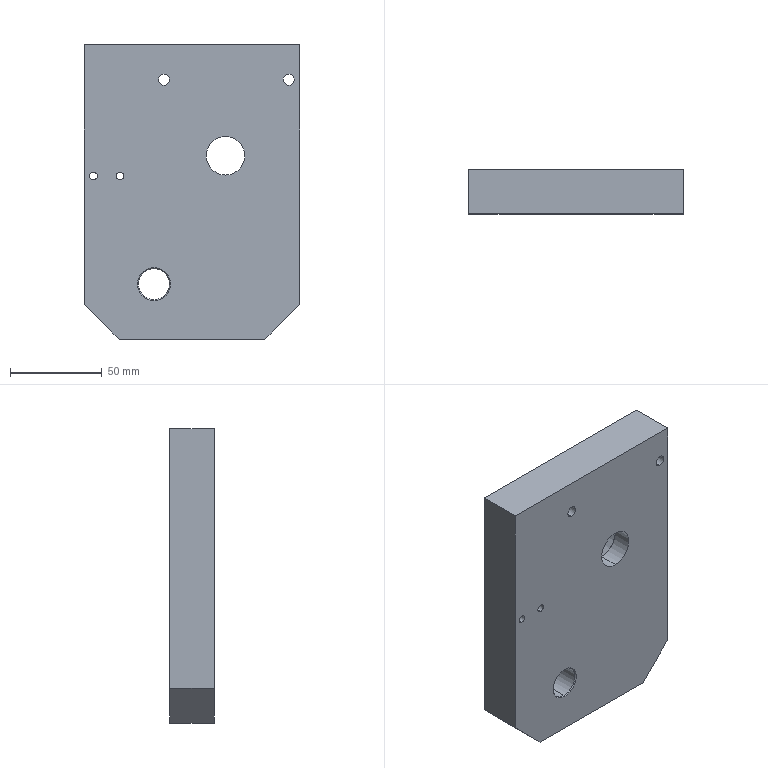Part | SolidWorks | features ICE 4, Chamfer 2, Extrusion 1, HoleWzd 1 | 1 solid | 44 faces | box 117.5 x 24 x 160.5 mm | volume 414919 mm3 | cylinder 17 | cone 14 | plane 13 | commonest cylinder face diameters 4.2 x4 6 x4 11 x3 17 x2 21 x2 40 x2
STEP:
#1=CARTESIAN_POINT('',(52.75,14.5,58.25));
#2=VERTEX_POINT('',#1);
#3=CARTESIAN_POINT('',(52.75,14.5,64.25));
#4=VERTEX_POINT('',#3);
#5=CARTESIAN_POINT('',(52.75,14.5,61.25));
#6=DIRECTION('',(0.,1.,0.));
#7=DIRECTION('',(0.,0.,1.));
#8=AXIS2_PLACEMENT_3D('',#5,#6,#7);
#9=CIRCLE('',#8,3.);
#10=EDGE_CURVE('',#2,#4,#9,.T.);
#11=ORIENTED_EDGE('',*,*,#10,.F.);
#12=CARTESIAN_POINT('',(52.75,15.,57.75));
#13=VERTEX_POINT('',#12);
#14=CARTESIAN_POINT('',(52.75,14.5,58.25));
#15=DIRECTION('',(0.,0.7071,-0.7071));
#16=VECTOR('',#15,1000.);
#17=LINE('',#14,#16);
#18=EDGE_CURVE('',#2,#13,#17,.T.);
#19=ORIENTED_EDGE('',*,*,#18,.T.);
#20=CARTESIAN_POINT('',(52.75,15.,64.75));
#21=VERTEX_POINT('',#20);
#22=CARTESIAN_POINT('',(52.75,15.,61.25));
#23=DIRECTION('',(0.,-1.,0.));
#24=DIRECTION('',(0.,0.,1.));
#25=AXIS2_PLACEMENT_3D('',#22,#23,#24);
#26=CIRCLE('',#25,3.5);
#27=EDGE_CURVE('',#21,#13,#26,.T.);
#28=ORIENTED_EDGE('',*,*,#27,.F.);
#29=CARTESIAN_POINT('',(52.75,14.5,64.25));
#30=DIRECTION('',(0.,0.7071,0.7071));
#31=VECTOR('',#30,1000.);
#32=LINE('',#29,#31);
#33=EDGE_CURVE('',#4,#21,#32,.T.);
#34=ORIENTED_EDGE('',*,*,#33,.F.);
#35=EDGE_LOOP('',(#11,#19,#28,#34));
#36=FACE_OUTER_BOUND('',#35,.T.);
#37=CARTESIAN_POINT('',(52.75,14.5,61.25));
#38=DIRECTION('',(0.,1.,0.));
#39=DIRECTION('',(0.,0.,1.));
#40=AXIS2_PLACEMENT_3D('',#37,#38,#39);
#41=CONICAL_SURFACE('',#40,3.,0.7854);
#42=ADVANCED_FACE('',(#36),#41,.F.);
#43=CARTESIAN_POINT('',(-15.25,15.,55.75));
#44=VERTEX_POINT('',#43);
#45=CARTESIAN_POINT('',(-15.25,15.,66.75));
#46=VERTEX_POINT('',#45);
#47=CARTESIAN_POINT('',(-15.25,15.,61.25));
#48=DIRECTION('',(0.,1.,0.));
#49=DIRECTION('',(0.,0.,1.));
#50=AXIS2_PLACEMENT_3D('',#47,#48,#49);
#51=CIRCLE('',#50,5.5);
#52=EDGE_CURVE('',#44,#46,#51,.T.);
#53=ORIENTED_EDGE('',*,*,#52,.F.);
#54=CARTESIAN_POINT('',(-15.25,24.,55.75));
#55=VERTEX_POINT('',#54);
#56=CARTESIAN_POINT('',(-15.25,15.,55.75));
#57=DIRECTION('',(0.,1.,0.));
#58=VECTOR('',#57,1000.);
#59=LINE('',#56,#58);
#60=EDGE_CURVE('',#44,#55,#59,.T.);
#61=ORIENTED_EDGE('',*,*,#60,.T.);
#62=CARTESIAN_POINT('',(-15.25,24.,66.75));
#63=VERTEX_POINT('',#62);
#64=CARTESIAN_POINT('',(-15.25,24.,61.25));
#65=DIRECTION('',(0.,1.,0.));
#66=DIRECTION('',(0.,0.,1.));
#67=AXIS2_PLACEMENT_3D('',#64,#65,#66);
#68=CIRCLE('',#67,5.5);
#69=EDGE_CURVE('',#55,#63,#68,.T.);
#70=ORIENTED_EDGE('',*,*,#69,.T.);
#71=CARTESIAN_POINT('',(-15.25,15.,66.75));
#72=DIRECTION('',(0.,1.,0.));
#73=VECTOR('',#72,1000.);
#74=LINE('',#71,#73);
#75=EDGE_CURVE('',#46,#63,#74,.T.);
#76=ORIENTED_EDGE('',*,*,#75,.F.);
#77=EDGE_LOOP('',(#53,#61,#70,#76));
#78=FACE_OUTER_BOUND('',#77,.T.);
#79=CARTESIAN_POINT('',(-15.25,15.,61.25));
#80=DIRECTION('',(0.,1.,0.));
#81=DIRECTION('',(0.,0.,1.));
#82=AXIS2_PLACEMENT_3D('',#79,#80,#81);
#83=CYLINDRICAL_SURFACE('',#82,5.5);
#84=ADVANCED_FACE('',(#78),#83,.F.);
#85=CARTESIAN_POINT('',(18.25,23.5,-0.25));
#86=VERTEX_POINT('',#85);
#87=CARTESIAN_POINT('',(18.25,23.5,39.75));
#88=VERTEX_POINT('',#87);
#89=CARTESIAN_POINT('',(18.25,23.5,19.75));
#90=DIRECTION('',(0.,1.,0.));
#91=DIRECTION('',(0.,0.,1.));
#92=AXIS2_PLACEMENT_3D('',#89,#90,#91);
#93=CIRCLE('',#92,20.);
#94=EDGE_CURVE('',#86,#88,#93,.T.);
#95=ORIENTED_EDGE('',*,*,#94,.F.);
#96=CARTESIAN_POINT('',(18.25,24.,-0.75));
#97=VERTEX_POINT('',#96);
#98=CARTESIAN_POINT('',(18.25,23.5,-0.25));
#99=DIRECTION('',(0.,0.7071,-0.7071));
#100=VECTOR('',#99,1000.);
#101=LINE('',#98,#100);
#102=EDGE_CURVE('',#86,#97,#101,.T.);
#103=ORIENTED_EDGE('',*,*,#102,.T.);
#104=CARTESIAN_POINT('',(18.25,24.,40.25));
#105=VERTEX_POINT('',#104);
#106=CARTESIAN_POINT('',(18.25,24.,19.75));
#107=DIRECTION('',(0.,-1.,0.));
#108=DIRECTION('',(0.,0.,1.));
#109=AXIS2_PLACEMENT_3D('',#106,#107,#108);
#110=CIRCLE('',#109,20.5);
#111=EDGE_CURVE('',#105,#97,#110,.T.);
#112=ORIENTED_EDGE('',*,*,#111,.F.);
#113=CARTESIAN_POINT('',(18.25,23.5,39.75));
#114=DIRECTION('',(0.,0.7071,0.7071));
#115=VECTOR('',#114,1000.);
#116=LINE('',#113,#115);
#117=EDGE_CURVE('',#88,#105,#116,.T.);
#118=ORIENTED_EDGE('',*,*,#117,.F.);
#119=EDGE_LOOP('',(#95,#103,#112,#118));
#120=FACE_OUTER_BOUND('',#119,.T.);
#121=CARTESIAN_POINT('',(18.25,23.5,19.75));
#122=DIRECTION('',(0.,1.,0.));
#123=DIRECTION('',(0.,0.,1.));
#124=AXIS2_PLACEMENT_3D('',#121,#122,#123);
#125=CONICAL_SURFACE('',#124,20.,0.7854);
#126=ADVANCED_FACE('',(#120),#125,.F.);
#127=CARTESIAN_POINT('',(18.25,10.5,9.25));
#128=VERTEX_POINT('',#127);
#129=CARTESIAN_POINT('',(18.25,10.5,30.25));
#130=VERTEX_POINT('',#129);
#131=CARTESIAN_POINT('',(18.25,10.5,19.75));
#132=DIRECTION('',(0.,1.,0.));
#133=DIRECTION('',(0.,0.,1.));
#134=AXIS2_PLACEMENT_3D('',#131,#132,#133);
#135=CIRCLE('',#134,10.5);
#136=EDGE_CURVE('',#128,#130,#135,.T.);
#137=ORIENTED_EDGE('',*,*,#136,.F.);
#138=CARTESIAN_POINT('',(18.25,11.,8.75));
#139=VERTEX_POINT('',#138);
#140=CARTESIAN_POINT('',(18.25,10.5,9.25));
#141=DIRECTION('',(0.,0.7071,-0.7071));
#142=VECTOR('',#141,1000.);
#143=LINE('',#140,#142);
#144=EDGE_CURVE('',#128,#139,#143,.T.);
#145=ORIENTED_EDGE('',*,*,#144,.T.);
#146=CARTESIAN_POINT('',(18.25,11.,30.75));
#147=VERTEX_POINT('',#146);
#148=CARTESIAN_POINT('',(18.25,11.,19.75));
#149=DIRECTION('',(0.,-1.,0.));
#150=DIRECTION('',(0.,0.,1.));
#151=AXIS2_PLACEMENT_3D('',#148,#149,#150);
#152=CIRCLE('',#151,11.);
#153=EDGE_CURVE('',#147,#139,#152,.T.);
#154=ORIENTED_EDGE('',*,*,#153,.F.);
#155=CARTESIAN_POINT('',(18.25,10.5,30.25));
#156=DIRECTION('',(0.,0.7071,0.7071));
#157=VECTOR('',#156,1000.);
#158=LINE('',#155,#157);
#159=EDGE_CURVE('',#130,#147,#158,.T.);
#160=ORIENTED_EDGE('',*,*,#159,.F.);
#161=EDGE_LOOP('',(#137,#145,#154,#160));
#162=FACE_OUTER_BOUND('',#161,.T.);
#163=CARTESIAN_POINT('',(18.25,10.5,19.75));
#164=DIRECTION('',(0.,1.,0.));
#165=DIRECTION('',(0.,0.,1.));
#166=AXIS2_PLACEMENT_3D('',#163,#164,#165);
#167=CONICAL_SURFACE('',#166,10.5,0.7854);
#168=ADVANCED_FACE('',(#162),#167,.F.);
#169=CARTESIAN_POINT('',(-20.75,23.5,-58.75));
#170=VERTEX_POINT('',#169);
#171=CARTESIAN_POINT('',(-20.75,23.5,-41.75));
#172=VERTEX_POINT('',#171);
#173=CARTESIAN_POINT('',(-20.75,23.5,-50.25));
#174=DIRECTION('',(0.,1.,0.));
#175=DIRECTION('',(0.,0.,1.));
#176=AXIS2_PLACEMENT_3D('',#173,#174,#175);
#177=CIRCLE('',#176,8.5);
#178=EDGE_CURVE('',#170,#172,#177,.T.);
#179=ORIENTED_EDGE('',*,*,#178,.F.);
#180=CARTESIAN_POINT('',(-20.75,24.,-59.25));
#181=VERTEX_POINT('',#180);
#182=CARTESIAN_POINT('',(-20.75,23.5,-58.75));
#183=DIRECTION('',(0.,0.7071,-0.7071));
#184=VECTOR('',#183,1000.);
#185=LINE('',#182,#184);
#186=EDGE_CURVE('',#170,#181,#185,.T.);
#187=ORIENTED_EDGE('',*,*,#186,.T.);
#188=CARTESIAN_POINT('',(-20.75,24.,-41.25));
#189=VERTEX_POINT('',#188);
#190=CARTESIAN_POINT('',(-20.75,24.,-50.25));
#191=DIRECTION('',(0.,-1.,0.));
#192=DIRECTION('',(0.,0.,1.));
#193=AXIS2_PLACEMENT_3D('',#190,#191,#192);
#194=CIRCLE('',#193,9.);
#195=EDGE_CURVE('',#189,#181,#194,.T.);
#196=ORIENTED_EDGE('',*,*,#195,.F.);
#197=CARTESIAN_POINT('',(-20.75,23.5,-41.75));
#198=DIRECTION('',(0.,0.7071,0.7071));
#199=VECTOR('',#198,1000.);
#200=LINE('',#197,#199);
#201=EDGE_CURVE('',#172,#189,#200,.T.);
#202=ORIENTED_EDGE('',*,*,#201,.F.);
#203=EDGE_LOOP('',(#179,#187,#196,#202));
#204=FACE_OUTER_BOUND('',#203,.T.);
#205=CARTESIAN_POINT('',(-20.75,23.5,-50.25));
#206=DIRECTION('',(0.,1.,0.));
#207=DIRECTION('',(0.,0.,1.));
#208=AXIS2_PLACEMENT_3D('',#205,#206,#207);
#209=CONICAL_SURFACE('',#208,8.5,0.7854);
#210=ADVANCED_FACE('',(#204),#209,.F.);
#211=CARTESIAN_POINT('',(-20.75,0.5,-41.75));
#212=VERTEX_POINT('',#211);
#213=CARTESIAN_POINT('',(-20.75,0.5,-58.75));
#214=VERTEX_POINT('',#213);
#215=CARTESIAN_POINT('',(-20.75,0.5,-50.25));
#216=DIRECTION('',(0.,-1.,0.));
#217=DIRECTION('',(0.,0.,1.));
#218=AXIS2_PLACEMENT_3D('',#215,#216,#217);
#219=CIRCLE('',#218,8.5);
#220=EDGE_CURVE('',#212,#214,#219,.T.);
#221=ORIENTED_EDGE('',*,*,#220,.F.);
#222=CARTESIAN_POINT('',(-20.75,0.,-41.25));
#223=VERTEX_POINT('',#222);
#224=CARTESIAN_POINT('',(-20.75,0.,-41.25));
#225=DIRECTION('',(0.,-0.7071,0.7071));
#226=VECTOR('',#225,1000.);
#227=LINE('',#224,#226);
#228=EDGE_CURVE('',#212,#223,#227,.T.);
#229=ORIENTED_EDGE('',*,*,#228,.T.);
#230=CARTESIAN_POINT('',(-20.75,0.,-59.25));
#231=VERTEX_POINT('',#230);
#232=CARTESIAN_POINT('',(-20.75,0.,-50.25));
#233=DIRECTION('',(0.,1.,0.));
#234=DIRECTION('',(0.,0.,1.));
#235=AXIS2_PLACEMENT_3D('',#232,#233,#234);
#236=CIRCLE('',#235,9.);
#237=EDGE_CURVE('',#231,#223,#236,.T.);
#238=ORIENTED_EDGE('',*,*,#237,.F.);
#239=CARTESIAN_POINT('',(-20.75,0.,-59.25));
#240=DIRECTION('',(0.,-0.7071,-0.7071));
#241=VECTOR('',#240,1000.);
#242=LINE('',#239,#241);
#243=EDGE_CURVE('',#214,#231,#242,.T.);
#244=ORIENTED_EDGE('',*,*,#243,.F.);
#245=EDGE_LOOP('',(#221,#229,#238,#244));
#246=FACE_OUTER_BOUND('',#245,.T.);
#247=CARTESIAN_POINT('',(-20.75,0.,-50.25));
#248=DIRECTION('',(0.,-1.,0.));
#249=DIRECTION('',(0.,0.,-1.));
#250=AXIS2_PLACEMENT_3D('',#247,#248,#249);
#251=CONICAL_SURFACE('',#250,9.,0.7854);
#252=ADVANCED_FACE('',(#246),#251,.F.);
#253=CARTESIAN_POINT('',(-53.75,23.575,6.65));
#254=VERTEX_POINT('',#253);
#255=CARTESIAN_POINT('',(-53.75,23.575,10.85));
#256=VERTEX_POINT('',#255);
#257=CARTESIAN_POINT('',(-53.75,23.575,8.75));
#258=DIRECTION('',(0.,1.,0.));
#259=DIRECTION('',(0.,0.,1.));
#260=AXIS2_PLACEMENT_3D('',#257,#258,#259);
#261=CIRCLE('',#260,2.1);
#262=EDGE_CURVE('',#254,#256,#261,.T.);
#263=ORIENTED_EDGE('',*,*,#262,.F.);
#264=CARTESIAN_POINT('',(-53.75,24.,6.225));
#265=VERTEX_POINT('',#264);
#266=CARTESIAN_POINT('',(-53.75,24.,6.225));
#267=DIRECTION('',(0.,0.7071,-0.7071));
#268=VECTOR('',#267,1000.);
#269=LINE('',#266,#268);
#270=EDGE_CURVE('',#254,#265,#269,.T.);
#271=ORIENTED_EDGE('',*,*,#270,.T.);
#272=CARTESIAN_POINT('',(-53.75,24.,11.275));
#273=VERTEX_POINT('',#272);
#274=CARTESIAN_POINT('',(-53.75,24.,8.75));
#275=DIRECTION('',(0.,1.,0.));
#276=DIRECTION('',(0.,0.,1.));
#277=AXIS2_PLACEMENT_3D('',#274,#275,#276);
#278=CIRCLE('',#277,2.525);
#279=EDGE_CURVE('',#265,#273,#278,.T.);
#280=ORIENTED_EDGE('',*,*,#279,.T.);
#281=CARTESIAN_POINT('',(-53.75,24.,11.275));
#282=DIRECTION('',(0.,0.7071,0.7071));
#283=VECTOR('',#282,1000.);
#284=LINE('',#281,#283);
#285=EDGE_CURVE('',#256,#273,#284,.T.);
#286=ORIENTED_EDGE('',*,*,#285,.F.);
#287=EDGE_LOOP('',(#263,#271,#280,#286));
#288=FACE_OUTER_BOUND('',#287,.T.);
#289=CARTESIAN_POINT('',(-53.75,24.,8.75));
#290=DIRECTION('',(0.,1.,0.));
#291=DIRECTION('',(0.,0.,1.));
#292=AXIS2_PLACEMENT_3D('',#289,#290,#291);
#293=CONICAL_SURFACE('',#292,2.525,0.7854);
#294=ADVANCED_FACE('',(#288),#293,.F.);
#295=CARTESIAN_POINT('',(-53.75,0.,6.65));
#296=VERTEX_POINT('',#295);
#297=CARTESIAN_POINT('',(-53.75,0.,10.85));
#298=VERTEX_POINT('',#297);
#299=CARTESIAN_POINT('',(-53.75,0.,8.75));
#300=DIRECTION('',(0.,1.,0.));
#301=DIRECTION('',(0.,0.,1.));
#302=AXIS2_PLACEMENT_3D('',#299,#300,#301);
#303=CIRCLE('',#302,2.1);
#304=EDGE_CURVE('',#296,#298,#303,.T.);
#305=ORIENTED_EDGE('',*,*,#304,.F.);
#306=CARTESIAN_POINT('',(-53.75,24.,6.65));
#307=DIRECTION('',(0.,1.,0.));
#308=VECTOR('',#307,1000.);
#309=LINE('',#306,#308);
#310=EDGE_CURVE('',#296,#254,#309,.T.);
#311=ORIENTED_EDGE('',*,*,#310,.T.);
#312=ORIENTED_EDGE('',*,*,#262,.T.);
#313=CARTESIAN_POINT('',(-53.75,24.,10.85));
#314=DIRECTION('',(0.,1.,0.));
#315=VECTOR('',#314,1000.);
#316=LINE('',#313,#315);
#317=EDGE_CURVE('',#298,#256,#316,.T.);
#318=ORIENTED_EDGE('',*,*,#317,.F.);
#319=EDGE_LOOP('',(#305,#311,#312,#318));
#320=FACE_OUTER_BOUND('',#319,.T.);
#321=CARTESIAN_POINT('',(-53.75,24.,8.75));
#322=DIRECTION('',(0.,1.,0.));
#323=DIRECTION('',(0.,0.,1.));
#324=AXIS2_PLACEMENT_3D('',#321,#322,#323);
#325=CYLINDRICAL_SURFACE('',#324,2.1);
#326=ADVANCED_FACE('',(#320),#325,.F.);
#327=CARTESIAN_POINT('',(-39.25,23.575,6.65));
#328=VERTEX_POINT('',#327);
#329=CARTESIAN_POINT('',(-39.25,23.575,10.85));
#330=VERTEX_POINT('',#329);
#331=CARTESIAN_POINT('',(-39.25,23.575,8.75));
#332=DIRECTION('',(0.,1.,0.));
#333=DIRECTION('',(0.,0.,1.));
#334=AXIS2_PLACEMENT_3D('',#331,#332,#333);
#335=CIRCLE('',#334,2.1);
#336=EDGE_CURVE('',#328,#330,#335,.T.);
#337=ORIENTED_EDGE('',*,*,#336,.F.);
#338=CARTESIAN_POINT('',(-39.25,24.,6.225));
#339=VERTEX_POINT('',#338);
#340=CARTESIAN_POINT('',(-39.25,24.,6.225));
#341=DIRECTION('',(0.,0.7071,-0.7071));
#342=VECTOR('',#341,1000.);
#343=LINE('',#340,#342);
#344=EDGE_CURVE('',#328,#339,#343,.T.);
#345=ORIENTED_EDGE('',*,*,#344,.T.);
#346=CARTESIAN_POINT('',(-39.25,24.,11.275));
#347=VERTEX_POINT('',#346);
#348=CARTESIAN_POINT('',(-39.25,24.,8.75));
#349=DIRECTION('',(0.,1.,0.));
#350=DIRECTION('',(0.,0.,1.));
#351=AXIS2_PLACEMENT_3D('',#348,#349,#350);
#352=CIRCLE('',#351,2.525);
#353=EDGE_CURVE('',#339,#347,#352,.T.);
#354=ORIENTED_EDGE('',*,*,#353,.T.);
#355=CARTESIAN_POINT('',(-39.25,24.,11.275));
#356=DIRECTION('',(0.,0.7071,0.7071));
#357=VECTOR('',#356,1000.);
#358=LINE('',#355,#357);
#359=EDGE_CURVE('',#330,#347,#358,.T.);
#360=ORIENTED_EDGE('',*,*,#359,.F.);
#361=EDGE_LOOP('',(#337,#345,#354,#360));
#362=FACE_OUTER_BOUND('',#361,.T.);
#363=CARTESIAN_POINT('',(-39.25,24.,8.75));
#364=DIRECTION('',(0.,1.,0.));
#365=DIRECTION('',(0.,0.,1.));
#366=AXIS2_PLACEMENT_3D('',#363,#364,#365);
#367=CONICAL_SURFACE('',#366,2.525,0.7854);
#368=ADVANCED_FACE('',(#362),#367,.F.);
#369=CARTESIAN_POINT('',(-39.25,0.,6.65));
#370=VERTEX_POINT('',#369);
#371=CARTESIAN_POINT('',(-39.25,0.,10.85));
#372=VERTEX_POINT('',#371);
#373=CARTESIAN_POINT('',(-39.25,0.,8.75));
#374=DIRECTION('',(0.,1.,0.));
#375=DIRECTION('',(0.,0.,1.));
#376=AXIS2_PLACEMENT_3D('',#373,#374,#375);
#377=CIRCLE('',#376,2.1);
#378=EDGE_CURVE('',#370,#372,#377,.T.);
#379=ORIENTED_EDGE('',*,*,#378,.F.);
#380=CARTESIAN_POINT('',(-39.25,24.,6.65));
#381=DIRECTION('',(0.,1.,0.));
#382=VECTOR('',#381,1000.);
#383=LINE('',#380,#382);
#384=EDGE_CURVE('',#370,#328,#383,.T.);
#385=ORIENTED_EDGE('',*,*,#384,.T.);
#386=ORIENTED_EDGE('',*,*,#336,.T.);
#387=CARTESIAN_POINT('',(-39.25,24.,10.85));
#388=DIRECTION('',(0.,1.,0.));
#389=VECTOR('',#388,1000.);
#390=LINE('',#387,#389);
#391=EDGE_CURVE('',#372,#330,#390,.T.);
#392=ORIENTED_EDGE('',*,*,#391,.F.);
#393=EDGE_LOOP('',(#379,#385,#386,#392));
#394=FACE_OUTER_BOUND('',#393,.T.);
#395=CARTESIAN_POINT('',(-39.25,24.,8.75));
#396=DIRECTION('',(0.,1.,0.));
#397=DIRECTION('',(0.,0.,1.));
#398=AXIS2_PLACEMENT_3D('',#395,#396,#397);
#399=CYLINDRICAL_SURFACE('',#398,2.1);
#400=ADVANCED_FACE('',(#394),#399,.F.);
#401=CARTESIAN_POINT('',(18.25,0.,9.25));
#402=VERTEX_POINT('',#401);
#403=CARTESIAN_POINT('',(18.25,0.,30.25));
#404=VERTEX_POINT('',#403);
#405=CARTESIAN_POINT('',(18.25,0.,19.75));
#406=DIRECTION('',(0.,1.,0.));
#407=DIRECTION('',(0.,0.,1.));
#408=AXIS2_PLACEMENT_3D('',#405,#406,#407);
#409=CIRCLE('',#408,10.5);
#410=EDGE_CURVE('',#402,#404,#409,.T.);
#411=ORIENTED_EDGE('',*,*,#410,.F.);
#412=CARTESIAN_POINT('',(18.25,0.,9.25));
#413=DIRECTION('',(0.,1.,0.));
#414=VECTOR('',#413,1000.);
#415=LINE('',#412,#414);
#416=EDGE_CURVE('',#402,#128,#415,.T.);
#417=ORIENTED_EDGE('',*,*,#416,.T.);
#418=ORIENTED_EDGE('',*,*,#136,.T.);
#419=CARTESIAN_POINT('',(18.25,0.,30.25));
#420=DIRECTION('',(0.,1.,0.));
#421=VECTOR('',#420,1000.);
#422=LINE('',#419,#421);
#423=EDGE_CURVE('',#404,#130,#422,.T.);
#424=ORIENTED_EDGE('',*,*,#423,.F.);
#425=EDGE_LOOP('',(#411,#417,#418,#424));
#426=FACE_OUTER_BOUND('',#425,.T.);
#427=CARTESIAN_POINT('',(18.25,0.,19.75));
#428=DIRECTION('',(0.,1.,0.));
#429=DIRECTION('',(0.,0.,1.));
#430=AXIS2_PLACEMENT_3D('',#427,#428,#429);
#431=CYLINDRICAL_SURFACE('',#430,10.5);
#432=ADVANCED_FACE('',(#426),#431,.F.);
#433=ORIENTED_EDGE('',*,*,#220,.T.);
#434=CARTESIAN_POINT('',(-20.75,11.,-58.75));
#435=DIRECTION('',(0.,1.,0.));
#436=VECTOR('',#435,1000.);
#437=LINE('',#434,#436);
#438=EDGE_CURVE('',#214,#170,#437,.T.);
#439=ORIENTED_EDGE('',*,*,#438,.T.);
#440=ORIENTED_EDGE('',*,*,#178,.T.);
#441=CARTESIAN_POINT('',(-20.75,11.,-41.75));
#442=DIRECTION('',(0.,1.,0.));
#443=VECTOR('',#442,1000.);
#444=LINE('',#441,#443);
#445=EDGE_CURVE('',#212,#172,#444,.T.);
#446=ORIENTED_EDGE('',*,*,#445,.F.);
#447=EDGE_LOOP('',(#433,#439,#440,#446));
#448=FACE_OUTER_BOUND('',#447,.T.);
#449=CARTESIAN_POINT('',(-20.75,11.,-50.25));
#450=DIRECTION('',(0.,1.,0.));
#451=DIRECTION('',(0.,0.,1.));
#452=AXIS2_PLACEMENT_3D('',#449,#450,#451);
#453=CYLINDRICAL_SURFACE('',#452,8.5);
#454=ADVANCED_FACE('',(#448),#453,.F.);
#455=CARTESIAN_POINT('',(18.25,11.,-0.25));
#456=VERTEX_POINT('',#455);
#457=CARTESIAN_POINT('',(18.25,11.,39.75));
#458=VERTEX_POINT('',#457);
#459=CARTESIAN_POINT('',(18.25,11.,19.75));
#460=DIRECTION('',(0.,1.,0.));
#461=DIRECTION('',(0.,0.,1.));
#462=AXIS2_PLACEMENT_3D('',#459,#460,#461);
#463=CIRCLE('',#462,20.);
#464=EDGE_CURVE('',#456,#458,#463,.T.);
#465=ORIENTED_EDGE('',*,*,#464,.F.);
#466=CARTESIAN_POINT('',(18.25,11.,-0.25));
#467=DIRECTION('',(0.,1.,0.));
#468=VECTOR('',#467,1000.);
#469=LINE('',#466,#468);
#470=EDGE_CURVE('',#456,#86,#469,.T.);
#471=ORIENTED_EDGE('',*,*,#470,.T.);
#472=ORIENTED_EDGE('',*,*,#94,.T.);
#473=CARTESIAN_POINT('',(18.25,11.,39.75));
#474=DIRECTION('',(0.,1.,0.));
#475=VECTOR('',#474,1000.);
#476=LINE('',#473,#475);
#477=EDGE_CURVE('',#458,#88,#476,.T.);
#478=ORIENTED_EDGE('',*,*,#477,.F.);
#479=EDGE_LOOP('',(#465,#471,#472,#478));
#480=FACE_OUTER_BOUND('',#479,.T.);
#481=CARTESIAN_POINT('',(18.25,11.,19.75));
#482=DIRECTION('',(0.,1.,0.));
#483=DIRECTION('',(0.,0.,1.));
#484=AXIS2_PLACEMENT_3D('',#481,#482,#483);
#485=CYLINDRICAL_SURFACE('',#484,20.);
#486=ADVANCED_FACE('',(#480),#485,.F.);
#487=CARTESIAN_POINT('',(52.75,0.,58.25));
#488=VERTEX_POINT('',#487);
#489=CARTESIAN_POINT('',(52.75,0.,64.25));
#490=VERTEX_POINT('',#489);
#491=CARTESIAN_POINT('',(52.75,0.,61.25));
#492=DIRECTION('',(0.,1.,0.));
#493=DIRECTION('',(0.,0.,1.));
#494=AXIS2_PLACEMENT_3D('',#491,#492,#493);
#495=CIRCLE('',#494,3.);
#496=EDGE_CURVE('',#488,#490,#495,.T.);
#497=ORIENTED_EDGE('',*,*,#496,.F.);
#498=CARTESIAN_POINT('',(52.75,11.,58.25));
#499=DIRECTION('',(0.,1.,0.));
#500=VECTOR('',#499,1000.);
#501=LINE('',#498,#500);
#502=EDGE_CURVE('',#488,#2,#501,.T.);
#503=ORIENTED_EDGE('',*,*,#502,.T.);
#504=ORIENTED_EDGE('',*,*,#10,.T.);
#505=CARTESIAN_POINT('',(52.75,11.,64.25));
#506=DIRECTION('',(0.,1.,0.));
#507=VECTOR('',#506,1000.);
#508=LINE('',#505,#507);
#509=EDGE_CURVE('',#490,#4,#508,.T.);
#510=ORIENTED_EDGE('',*,*,#509,.F.);
#511=EDGE_LOOP('',(#497,#503,#504,#510));
#512=FACE_OUTER_BOUND('',#511,.T.);
#513=CARTESIAN_POINT('',(52.75,11.,61.25));
#514=DIRECTION('',(0.,1.,0.));
#515=DIRECTION('',(0.,0.,1.));
#516=AXIS2_PLACEMENT_3D('',#513,#514,#515);
#517=CYLINDRICAL_SURFACE('',#516,3.);
#518=ADVANCED_FACE('',(#512),#517,.F.);
#519=CARTESIAN_POINT('',(-15.25,0.,58.25));
#520=VERTEX_POINT('',#519);
#521=CARTESIAN_POINT('',(-15.25,0.,64.25));
#522=VERTEX_POINT('',#521);
#523=CARTESIAN_POINT('',(-15.25,0.,61.25));
#524=DIRECTION('',(0.,1.,0.));
#525=DIRECTION('',(0.,0.,1.));
#526=AXIS2_PLACEMENT_3D('',#523,#524,#525);
#527=CIRCLE('',#526,3.);
#528=EDGE_CURVE('',#520,#522,#527,.T.);
#529=ORIENTED_EDGE('',*,*,#528,.F.);
#530=CARTESIAN_POINT('',(-15.25,15.,58.25));
#531=VERTEX_POINT('',#530);
#532=CARTESIAN_POINT('',(-15.25,11.,58.25));
#533=DIRECTION('',(0.,1.,0.));
#534=VECTOR('',#533,1000.);
#535=LINE('',#532,#534);
#536=EDGE_CURVE('',#520,#531,#535,.T.);
#537=ORIENTED_EDGE('',*,*,#536,.T.);
#538=CARTESIAN_POINT('',(-15.25,15.,64.25));
#539=VERTEX_POINT('',#538);
#540=CARTESIAN_POINT('',(-15.25,15.,61.25));
#541=DIRECTION('',(0.,1.,0.));
#542=DIRECTION('',(0.,0.,1.));
#543=AXIS2_PLACEMENT_3D('',#540,#541,#542);
#544=CIRCLE('',#543,3.);
#545=EDGE_CURVE('',#531,#539,#544,.T.);
#546=ORIENTED_EDGE('',*,*,#545,.T.);
#547=CARTESIAN_POINT('',(-15.25,11.,64.25));
#548=DIRECTION('',(0.,1.,0.));
#549=VECTOR('',#548,1000.);
#550=LINE('',#547,#549);
#551=EDGE_CURVE('',#522,#539,#550,.T.);
#552=ORIENTED_EDGE('',*,*,#551,.F.);
#553=EDGE_LOOP('',(#529,#537,#546,#552));
#554=FACE_OUTER_BOUND('',#553,.T.);
#555=CARTESIAN_POINT('',(-15.25,11.,61.25));
#556=DIRECTION('',(0.,1.,0.));
#557=DIRECTION('',(0.,0.,1.));
#558=AXIS2_PLACEMENT_3D('',#555,#556,#557);
#559=CYLINDRICAL_SURFACE('',#558,3.);
#560=ADVANCED_FACE('',(#554),#559,.F.);
#561=CARTESIAN_POINT('',(58.75,24.,66.75));
#562=VERTEX_POINT('',#561);
#563=CARTESIAN_POINT('',(58.75,15.,66.75));
#564=VERTEX_POINT('',#563);
#565=CARTESIAN_POINT('',(58.75,24.,66.75));
#566=DIRECTION('',(0.,-1.,0.));
#567=VECTOR('',#566,1000.);
#568=LINE('',#565,#567);
#569=EDGE_CURVE('',#562,#564,#568,.T.);
#570=ORIENTED_EDGE('',*,*,#569,.F.);
#571=CARTESIAN_POINT('',(58.75,24.,80.25));
#572=VERTEX_POINT('',#571);
#573=CARTESIAN_POINT('',(58.75,24.,-61.25));
#574=DIRECTION('',(0.,0.,-1.));
#575=VECTOR('',#574,1000.);
#576=LINE('',#573,#575);
#577=EDGE_CURVE('',#572,#562,#576,.T.);
#578=ORIENTED_EDGE('',*,*,#577,.F.);
#579=CARTESIAN_POINT('',(58.75,0.,80.25));
#580=VERTEX_POINT('',#579);
#581=CARTESIAN_POINT('',(58.75,24.,80.25));
#582=DIRECTION('',(0.,-1.,0.));
#583=VECTOR('',#582,1000.);
#584=LINE('',#581,#583);
#585=EDGE_CURVE('',#572,#580,#584,.T.);
#586=ORIENTED_EDGE('',*,*,#585,.T.);
#587=CARTESIAN_POINT('',(58.75,0.,-61.25));
#588=VERTEX_POINT('',#587);
#589=CARTESIAN_POINT('',(58.75,0.,-61.25));
#590=DIRECTION('',(0.,0.,-1.));
#591=VECTOR('',#590,1000.);
#592=LINE('',#589,#591);
#593=EDGE_CURVE('',#580,#588,#592,.T.);
#594=ORIENTED_EDGE('',*,*,#593,.T.);
#595=CARTESIAN_POINT('',(58.75,24.,-61.25));
#596=VERTEX_POINT('',#595);
#597=CARTESIAN_POINT('',(58.75,24.,-61.25));
#598=DIRECTION('',(0.,-1.,0.));
#599=VECTOR('',#598,1000.);
#600=LINE('',#597,#599);
#601=EDGE_CURVE('',#596,#588,#600,.T.);
#602=ORIENTED_EDGE('',*,*,#601,.F.);
#603=CARTESIAN_POINT('',(58.75,24.,55.75));
#604=VERTEX_POINT('',#603);
#605=CARTESIAN_POINT('',(58.75,24.,-61.25));
#606=DIRECTION('',(0.,0.,-1.));
#607=VECTOR('',#606,1000.);
#608=LINE('',#605,#607);
#609=EDGE_CURVE('',#604,#596,#608,.T.);
#610=ORIENTED_EDGE('',*,*,#609,.F.);
#611=CARTESIAN_POINT('',(58.75,15.,55.75));
#612=VERTEX_POINT('',#611);
#613=CARTESIAN_POINT('',(58.75,24.,55.75));
#614=DIRECTION('',(0.,-1.,0.));
#615=VECTOR('',#614,1000.);
#616=LINE('',#613,#615);
#617=EDGE_CURVE('',#604,#612,#616,.T.);
#618=ORIENTED_EDGE('',*,*,#617,.T.);
#619=CARTESIAN_POINT('',(58.75,15.,-61.25));
#620=DIRECTION('',(0.,0.,-1.));
#621=VECTOR('',#620,1000.);
#622=LINE('',#619,#621);
#623=EDGE_CURVE('',#564,#612,#622,.T.);
#624=ORIENTED_EDGE('',*,*,#623,.F.);
#625=EDGE_LOOP('',(#570,#578,#586,#594,#602,#610,#618,#624));
#626=FACE_OUTER_BOUND('',#625,.T.);
#627=CARTESIAN_POINT('',(58.75,24.,-61.25));
#628=DIRECTION('',(-1.,0.,0.));
#629=DIRECTION('',(0.,0.,1.));
#630=AXIS2_PLACEMENT_3D('',#627,#628,#629);
#631=PLANE('',#630);
#632=ADVANCED_FACE('',(#626),#631,.F.);
#633=CARTESIAN_POINT('',(-15.25,24.,61.25));
#634=DIRECTION('',(0.,1.,0.));
#635=DIRECTION('',(0.,0.,1.));
#636=AXIS2_PLACEMENT_3D('',#633,#634,#635);
#637=CIRCLE('',#636,5.5);
#638=EDGE_CURVE('',#63,#55,#637,.T.);
#639=ORIENTED_EDGE('',*,*,#638,.F.);
#640=ORIENTED_EDGE('',*,*,#69,.F.);
#641=EDGE_LOOP('',(#639,#640));
#642=FACE_BOUND('',#641,.T.);
#643=CARTESIAN_POINT('',(-39.25,24.,8.75));
#644=DIRECTION('',(0.,1.,0.));
#645=DIRECTION('',(0.,0.,1.));
#646=AXIS2_PLACEMENT_3D('',#643,#644,#645);
#647=CIRCLE('',#646,2.525);
#648=EDGE_CURVE('',#347,#339,#647,.T.);
#649=ORIENTED_EDGE('',*,*,#648,.F.);
#650=ORIENTED_EDGE('',*,*,#353,.F.);
#651=EDGE_LOOP('',(#649,#650));
#652=FACE_BOUND('',#651,.T.);
#653=CARTESIAN_POINT('',(-53.75,24.,8.75));
#654=DIRECTION('',(0.,1.,0.));
#655=DIRECTION('',(0.,0.,1.));
#656=AXIS2_PLACEMENT_3D('',#653,#654,#655);
#657=CIRCLE('',#656,2.525);
#658=EDGE_CURVE('',#273,#265,#657,.T.);
#659=ORIENTED_EDGE('',*,*,#658,.F.);
#660=ORIENTED_EDGE('',*,*,#279,.F.);
#661=EDGE_LOOP('',(#659,#660));
#662=FACE_BOUND('',#661,.T.);
#663=ORIENTED_EDGE('',*,*,#111,.T.);
#664=CARTESIAN_POINT('',(18.25,24.,19.75));
#665=DIRECTION('',(0.,-1.,0.));
#666=DIRECTION('',(0.,0.,1.));
#667=AXIS2_PLACEMENT_3D('',#664,#665,#666);
#668=CIRCLE('',#667,20.5);
#669=EDGE_CURVE('',#97,#105,#668,.T.);
#670=ORIENTED_EDGE('',*,*,#669,.T.);
#671=EDGE_LOOP('',(#663,#670));
#672=FACE_BOUND('',#671,.T.);
#673=ORIENTED_EDGE('',*,*,#195,.T.);
#674=CARTESIAN_POINT('',(-20.75,24.,-50.25));
#675=DIRECTION('',(0.,-1.,0.));
#676=DIRECTION('',(0.,0.,1.));
#677=AXIS2_PLACEMENT_3D('',#674,#675,#676);
#678=CIRCLE('',#677,9.);
#679=EDGE_CURVE('',#181,#189,#678,.T.);
#680=ORIENTED_EDGE('',*,*,#679,.T.);
#681=EDGE_LOOP('',(#673,#680));
#682=FACE_BOUND('',#681,.T.);
#683=ORIENTED_EDGE('',*,*,#577,.T.);
#684=CARTESIAN_POINT('',(52.75,24.,66.75));
#685=VERTEX_POINT('',#684);
#686=CARTESIAN_POINT('',(0.,24.,66.75));
#687=DIRECTION('',(-1.,0.,0.));
#688=VECTOR('',#687,1000.);
#689=LINE('',#686,#688);
#690=EDGE_CURVE('',#562,#685,#689,.T.);
#691=ORIENTED_EDGE('',*,*,#690,.T.);
#692=CARTESIAN_POINT('',(52.75,24.,55.75));
#693=VERTEX_POINT('',#692);
#694=CARTESIAN_POINT('',(52.75,24.,61.25));
#695=DIRECTION('',(0.,1.,0.));
#696=DIRECTION('',(0.,0.,1.));
#697=AXIS2_PLACEMENT_3D('',#694,#695,#696);
#698=CIRCLE('',#697,5.5);
#699=EDGE_CURVE('',#693,#685,#698,.T.);
#700=ORIENTED_EDGE('',*,*,#699,.F.);
#701=CARTESIAN_POINT('',(0.,24.,55.75));
#702=DIRECTION('',(-1.,0.,0.));
#703=VECTOR('',#702,1000.);
#704=LINE('',#701,#703);
#705=EDGE_CURVE('',#604,#693,#704,.T.);
#706=ORIENTED_EDGE('',*,*,#705,.F.);
#707=ORIENTED_EDGE('',*,*,#609,.T.);
#708=CARTESIAN_POINT('',(39.75,24.,-80.25));
#709=VERTEX_POINT('',#708);
#710=CARTESIAN_POINT('',(39.75,24.,-80.25));
#711=DIRECTION('',(-0.7071,0.,-0.7071));
#712=VECTOR('',#711,1000.);
#713=LINE('',#710,#712);
#714=EDGE_CURVE('',#596,#709,#713,.T.);
#715=ORIENTED_EDGE('',*,*,#714,.T.);
#716=CARTESIAN_POINT('',(-39.75,24.,-80.25));
#717=VERTEX_POINT('',#716);
#718=CARTESIAN_POINT('',(-39.75,24.,-80.25));
#719=DIRECTION('',(-1.,0.,0.));
#720=VECTOR('',#719,1000.);
#721=LINE('',#718,#720);
#722=EDGE_CURVE('',#709,#717,#721,.T.);
#723=ORIENTED_EDGE('',*,*,#722,.T.);
#724=CARTESIAN_POINT('',(-58.75,24.,-61.25));
#725=VERTEX_POINT('',#724);
#726=CARTESIAN_POINT('',(-58.75,24.,-61.25));
#727=DIRECTION('',(-0.7071,0.,0.7071));
#728=VECTOR('',#727,1000.);
#729=LINE('',#726,#728);
#730=EDGE_CURVE('',#717,#725,#729,.T.);
#731=ORIENTED_EDGE('',*,*,#730,.T.);
#732=CARTESIAN_POINT('',(-58.75,24.,80.25));
#733=VERTEX_POINT('',#732);
#734=CARTESIAN_POINT('',(-58.75,24.,-61.25));
#735=DIRECTION('',(0.,0.,1.));
#736=VECTOR('',#735,1000.);
#737=LINE('',#734,#736);
#738=EDGE_CURVE('',#725,#733,#737,.T.);
#739=ORIENTED_EDGE('',*,*,#738,.T.);
#740=CARTESIAN_POINT('',(-58.75,24.,80.25));
#741=DIRECTION('',(1.,0.,0.));
#742=VECTOR('',#741,1000.);
#743=LINE('',#740,#742);
#744=EDGE_CURVE('',#733,#572,#743,.T.);
#745=ORIENTED_EDGE('',*,*,#744,.T.);
#746=EDGE_LOOP('',(#683,#691,#700,#706,#707,#715,#723,#731,#739,#745));
#747=FACE_OUTER_BOUND('',#746,.T.);
#748=CARTESIAN_POINT('',(0.,24.,0.));
#749=DIRECTION('',(0.,1.,0.));
#750=DIRECTION('',(0.,0.,1.));
#751=AXIS2_PLACEMENT_3D('',#748,#749,#750);
#752=PLANE('',#751);
#753=ADVANCED_FACE('',(#642,#652,#662,#672,#682,#747),#752,.T.);
#754=ORIENTED_EDGE('',*,*,#536,.F.);
#755=CARTESIAN_POINT('',(-15.25,0.,61.25));
#756=DIRECTION('',(0.,1.,0.));
#757=DIRECTION('',(0.,0.,1.));
#758=AXIS2_PLACEMENT_3D('',#755,#756,#757);
#759=CIRCLE('',#758,3.);
#760=EDGE_CURVE('',#522,#520,#759,.T.);
#761=ORIENTED_EDGE('',*,*,#760,.F.);
#762=ORIENTED_EDGE('',*,*,#551,.T.);
#763=CARTESIAN_POINT('',(-15.25,15.,61.25));
#764=DIRECTION('',(0.,1.,0.));
#765=DIRECTION('',(0.,0.,1.));
#766=AXIS2_PLACEMENT_3D('',#763,#764,#765);
#767=CIRCLE('',#766,3.);
#768=EDGE_CURVE('',#539,#531,#767,.T.);
#769=ORIENTED_EDGE('',*,*,#768,.T.);
#770=EDGE_LOOP('',(#754,#761,#762,#769));
#771=FACE_OUTER_BOUND('',#770,.T.);
#772=CARTESIAN_POINT('',(-15.25,11.,61.25));
#773=DIRECTION('',(0.,1.,0.));
#774=DIRECTION('',(0.,0.,1.));
#775=AXIS2_PLACEMENT_3D('',#772,#773,#774);
#776=CYLINDRICAL_SURFACE('',#775,3.);
#777=ADVANCED_FACE('',(#771),#776,.F.);
#778=ORIENTED_EDGE('',*,*,#502,.F.);
#779=CARTESIAN_POINT('',(52.75,0.,61.25));
#780=DIRECTION('',(0.,1.,0.));
#781=DIRECTION('',(0.,0.,1.));
#782=AXIS2_PLACEMENT_3D('',#779,#780,#781);
#783=CIRCLE('',#782,3.);
#784=EDGE_CURVE('',#490,#488,#783,.T.);
#785=ORIENTED_EDGE('',*,*,#784,.F.);
#786=ORIENTED_EDGE('',*,*,#509,.T.);
#787=CARTESIAN_POINT('',(52.75,14.5,61.25));
#788=DIRECTION('',(0.,1.,0.));
#789=DIRECTION('',(0.,0.,1.));
#790=AXIS2_PLACEMENT_3D('',#787,#788,#789);
#791=CIRCLE('',#790,3.);
#792=EDGE_CURVE('',#4,#2,#791,.T.);
#793=ORIENTED_EDGE('',*,*,#792,.T.);
#794=EDGE_LOOP('',(#778,#785,#786,#793));
#795=FACE_OUTER_BOUND('',#794,.T.);
#796=CARTESIAN_POINT('',(52.75,11.,61.25));
#797=DIRECTION('',(0.,1.,0.));
#798=DIRECTION('',(0.,0.,1.));
#799=AXIS2_PLACEMENT_3D('',#796,#797,#798);
#800=CYLINDRICAL_SURFACE('',#799,3.);
#801=ADVANCED_FACE('',(#795),#800,.F.);
#802=CARTESIAN_POINT('',(39.75,0.,-80.25));
#803=VERTEX_POINT('',#802);
#804=CARTESIAN_POINT('',(39.75,0.,-80.25));
#805=DIRECTION('',(-0.7071,0.,-0.7071));
#806=VECTOR('',#805,1000.);
#807=LINE('',#804,#806);
#808=EDGE_CURVE('',#588,#803,#807,.T.);
#809=ORIENTED_EDGE('',*,*,#808,.T.);
#810=CARTESIAN_POINT('',(39.75,24.,-80.25));
#811=DIRECTION('',(0.,-1.,0.));
#812=VECTOR('',#811,1000.);
#813=LINE('',#810,#812);
#814=EDGE_CURVE('',#709,#803,#813,.T.);
#815=ORIENTED_EDGE('',*,*,#814,.F.);
#816=ORIENTED_EDGE('',*,*,#714,.F.);
#817=ORIENTED_EDGE('',*,*,#601,.T.);
#818=EDGE_LOOP('',(#809,#815,#816,#817));
#819=FACE_OUTER_BOUND('',#818,.T.);
#820=CARTESIAN_POINT('',(39.75,24.,-80.25));
#821=DIRECTION('',(-0.7071,0.,0.7071));
#822=DIRECTION('',(0.7071,0.,0.7071));
#823=AXIS2_PLACEMENT_3D('',#820,#821,#822);
#824=PLANE('',#823);
#825=ADVANCED_FACE('',(#819),#824,.F.);
#826=CARTESIAN_POINT('',(-39.75,0.,-80.25));
#827=VERTEX_POINT('',#826);
#828=CARTESIAN_POINT('',(-39.75,0.,-80.25));
#829=DIRECTION('',(-1.,0.,0.));
#830=VECTOR('',#829,1000.);
#831=LINE('',#828,#830);
#832=EDGE_CURVE('',#803,#827,#831,.T.);
#833=ORIENTED_EDGE('',*,*,#832,.T.);
#834=CARTESIAN_POINT('',(-39.75,24.,-80.25));
#835=DIRECTION('',(0.,-1.,0.));
#836=VECTOR('',#835,1000.);
#837=LINE('',#834,#836);
#838=EDGE_CURVE('',#717,#827,#837,.T.);
#839=ORIENTED_EDGE('',*,*,#838,.F.);
#840=ORIENTED_EDGE('',*,*,#722,.F.);
#841=ORIENTED_EDGE('',*,*,#814,.T.);
#842=EDGE_LOOP('',(#833,#839,#840,#841));
#843=FACE_OUTER_BOUND('',#842,.T.);
#844=CARTESIAN_POINT('',(-39.75,24.,-80.25));
#845=DIRECTION('',(0.,0.,1.));
#846=DIRECTION('',(1.,0.,0.));
#847=AXIS2_PLACEMENT_3D('',#844,#845,#846);
#848=PLANE('',#847);
#849=ADVANCED_FACE('',(#843),#848,.F.);
#850=CARTESIAN_POINT('',(-58.75,0.,-61.25));
#851=VERTEX_POINT('',#850);
#852=CARTESIAN_POINT('',(-58.75,0.,-61.25));
#853=DIRECTION('',(-0.7071,0.,0.7071));
#854=VECTOR('',#853,1000.);
#855=LINE('',#852,#854);
#856=EDGE_CURVE('',#827,#851,#855,.T.);
#857=ORIENTED_EDGE('',*,*,#856,.T.);
#858=CARTESIAN_POINT('',(-58.75,24.,-61.25));
#859=DIRECTION('',(0.,-1.,0.));
#860=VECTOR('',#859,1000.);
#861=LINE('',#858,#860);
#862=EDGE_CURVE('',#725,#851,#861,.T.);
#863=ORIENTED_EDGE('',*,*,#862,.F.);
#864=ORIENTED_EDGE('',*,*,#730,.F.);
#865=ORIENTED_EDGE('',*,*,#838,.T.);
#866=EDGE_LOOP('',(#857,#863,#864,#865));
#867=FACE_OUTER_BOUND('',#866,.T.);
#868=CARTESIAN_POINT('',(-58.75,24.,-61.25));
#869=DIRECTION('',(0.7071,0.,0.7071));
#870=DIRECTION('',(0.7071,0.,-0.7071));
#871=AXIS2_PLACEMENT_3D('',#868,#869,#870);
#872=PLANE('',#871);
#873=ADVANCED_FACE('',(#867),#872,.F.);
#874=CARTESIAN_POINT('',(-58.75,0.,80.25));
#875=VERTEX_POINT('',#874);
#876=CARTESIAN_POINT('',(-58.75,0.,-61.25));
#877=DIRECTION('',(0.,0.,1.));
#878=VECTOR('',#877,1000.);
#879=LINE('',#876,#878);
#880=EDGE_CURVE('',#851,#875,#879,.T.);
#881=ORIENTED_EDGE('',*,*,#880,.T.);
#882=CARTESIAN_POINT('',(-58.75,24.,80.25));
#883=DIRECTION('',(0.,-1.,0.));
#884=VECTOR('',#883,1000.);
#885=LINE('',#882,#884);
#886=EDGE_CURVE('',#733,#875,#885,.T.);
#887=ORIENTED_EDGE('',*,*,#886,.F.);
#888=ORIENTED_EDGE('',*,*,#738,.F.);
#889=ORIENTED_EDGE('',*,*,#862,.T.);
#890=EDGE_LOOP('',(#881,#887,#888,#889));
#891=FACE_OUTER_BOUND('',#890,.T.);
#892=CARTESIAN_POINT('',(-58.75,24.,-61.25));
#893=DIRECTION('',(1.,0.,0.));
#894=DIRECTION('',(0.,0.,-1.));
#895=AXIS2_PLACEMENT_3D('',#892,#893,#894);
#896=PLANE('',#895);
#897=ADVANCED_FACE('',(#891),#896,.F.);
#898=CARTESIAN_POINT('',(-58.75,0.,80.25));
#899=DIRECTION('',(1.,0.,0.));
#900=VECTOR('',#899,1000.);
#901=LINE('',#898,#900);
#902=EDGE_CURVE('',#875,#580,#901,.T.);
#903=ORIENTED_EDGE('',*,*,#902,.T.);
#904=ORIENTED_EDGE('',*,*,#585,.F.);
#905=ORIENTED_EDGE('',*,*,#744,.F.);
#906=ORIENTED_EDGE('',*,*,#886,.T.);
#907=EDGE_LOOP('',(#903,#904,#905,#906));
#908=FACE_OUTER_BOUND('',#907,.T.);
#909=CARTESIAN_POINT('',(-58.75,24.,80.25));
#910=DIRECTION('',(0.,0.,-1.));
#911=DIRECTION('',(-1.,0.,0.));
#912=AXIS2_PLACEMENT_3D('',#909,#910,#911);
#913=PLANE('',#912);
#914=ADVANCED_FACE('',(#908),#913,.F.);
#915=ORIENTED_EDGE('',*,*,#237,.T.);
#916=CARTESIAN_POINT('',(-20.75,0.,-50.25));
#917=DIRECTION('',(0.,1.,0.));
#918=DIRECTION('',(0.,0.,1.));
#919=AXIS2_PLACEMENT_3D('',#916,#917,#918);
#920=CIRCLE('',#919,9.);
#921=EDGE_CURVE('',#223,#231,#920,.T.);
#922=ORIENTED_EDGE('',*,*,#921,.T.);
#923=EDGE_LOOP('',(#915,#922));
#924=FACE_BOUND('',#923,.T.);
#925=CARTESIAN_POINT('',(-53.75,0.,8.75));
#926=DIRECTION('',(0.,1.,0.));
#927=DIRECTION('',(0.,0.,1.));
#928=AXIS2_PLACEMENT_3D('',#925,#926,#927);
#929=CIRCLE('',#928,2.1);
#930=EDGE_CURVE('',#298,#296,#929,.T.);
#931=ORIENTED_EDGE('',*,*,#930,.T.);
#932=ORIENTED_EDGE('',*,*,#304,.T.);
#933=EDGE_LOOP('',(#931,#932));
#934=FACE_BOUND('',#933,.T.);
#935=CARTESIAN_POINT('',(-39.25,0.,8.75));
#936=DIRECTION('',(0.,1.,0.));
#937=DIRECTION('',(0.,0.,1.));
#938=AXIS2_PLACEMENT_3D('',#935,#936,#937);
#939=CIRCLE('',#938,2.1);
#940=EDGE_CURVE('',#372,#370,#939,.T.);
#941=ORIENTED_EDGE('',*,*,#940,.T.);
#942=ORIENTED_EDGE('',*,*,#378,.T.);
#943=EDGE_LOOP('',(#941,#942));
#944=FACE_BOUND('',#943,.T.);
#945=CARTESIAN_POINT('',(18.25,0.,19.75));
#946=DIRECTION('',(0.,1.,0.));
#947=DIRECTION('',(0.,0.,1.));
#948=AXIS2_PLACEMENT_3D('',#945,#946,#947);
#949=CIRCLE('',#948,10.5);
#950=EDGE_CURVE('',#404,#402,#949,.T.);
#951=ORIENTED_EDGE('',*,*,#950,.T.);
#952=ORIENTED_EDGE('',*,*,#410,.T.);
#953=EDGE_LOOP('',(#951,#952));
#954=FACE_BOUND('',#953,.T.);
#955=ORIENTED_EDGE('',*,*,#784,.T.);
#956=ORIENTED_EDGE('',*,*,#496,.T.);
#957=EDGE_LOOP('',(#955,#956));
#958=FACE_BOUND('',#957,.T.);
#959=ORIENTED_EDGE('',*,*,#760,.T.);
#960=ORIENTED_EDGE('',*,*,#528,.T.);
#961=EDGE_LOOP('',(#959,#960));
#962=FACE_BOUND('',#961,.T.);
#963=ORIENTED_EDGE('',*,*,#593,.F.);
#964=ORIENTED_EDGE('',*,*,#902,.F.);
#965=ORIENTED_EDGE('',*,*,#880,.F.);
#966=ORIENTED_EDGE('',*,*,#856,.F.);
#967=ORIENTED_EDGE('',*,*,#832,.F.);
#968=ORIENTED_EDGE('',*,*,#808,.F.);
#969=EDGE_LOOP('',(#963,#964,#965,#966,#967,#968));
#970=FACE_OUTER_BOUND('',#969,.T.);
#971=CARTESIAN_POINT('',(0.,0.,0.));
#972=DIRECTION('',(0.,1.,0.));
#973=DIRECTION('',(0.,0.,1.));
#974=AXIS2_PLACEMENT_3D('',#971,#972,#973);
#975=PLANE('',#974);
#976=ADVANCED_FACE('',(#924,#934,#944,#954,#958,#962,#970),#975,.F.);
#977=ORIENTED_EDGE('',*,*,#470,.F.);
#978=CARTESIAN_POINT('',(18.25,11.,19.75));
#979=DIRECTION('',(0.,1.,0.));
#980=DIRECTION('',(0.,0.,1.));
#981=AXIS2_PLACEMENT_3D('',#978,#979,#980);
#982=CIRCLE('',#981,20.);
#983=EDGE_CURVE('',#458,#456,#982,.T.);
#984=ORIENTED_EDGE('',*,*,#983,.F.);
#985=ORIENTED_EDGE('',*,*,#477,.T.);
#986=CARTESIAN_POINT('',(18.25,23.5,19.75));
#987=DIRECTION('',(0.,1.,0.));
#988=DIRECTION('',(0.,0.,1.));
#989=AXIS2_PLACEMENT_3D('',#986,#987,#988);
#990=CIRCLE('',#989,20.);
#991=EDGE_CURVE('',#88,#86,#990,.T.);
#992=ORIENTED_EDGE('',*,*,#991,.T.);
#993=EDGE_LOOP('',(#977,#984,#985,#992));
#994=FACE_OUTER_BOUND('',#993,.T.);
#995=CARTESIAN_POINT('',(18.25,11.,19.75));
#996=DIRECTION('',(0.,1.,0.));
#997=DIRECTION('',(0.,0.,1.));
#998=AXIS2_PLACEMENT_3D('',#995,#996,#997);
#999=CYLINDRICAL_SURFACE('',#998,20.);
#1000=ADVANCED_FACE('',(#994),#999,.F.);
#1001=ORIENTED_EDGE('',*,*,#153,.T.);
#1002=CARTESIAN_POINT('',(18.25,11.,19.75));
#1003=DIRECTION('',(0.,-1.,0.));
#1004=DIRECTION('',(0.,0.,1.));
#1005=AXIS2_PLACEMENT_3D('',#1002,#1003,#1004);
#1006=CIRCLE('',#1005,11.);
#1007=EDGE_CURVE('',#139,#147,#1006,.T.);
#1008=ORIENTED_EDGE('',*,*,#1007,.T.);
#1009=EDGE_LOOP('',(#1001,#1008));
#1010=FACE_BOUND('',#1009,.T.);
#1011=ORIENTED_EDGE('',*,*,#983,.T.);
#1012=ORIENTED_EDGE('',*,*,#464,.T.);
#1013=EDGE_LOOP('',(#1011,#1012));
#1014=FACE_OUTER_BOUND('',#1013,.T.);
#1015=CARTESIAN_POINT('',(18.25,11.,19.75));
#1016=DIRECTION('',(0.,1.,0.));
#1017=DIRECTION('',(0.,0.,1.));
#1018=AXIS2_PLACEMENT_3D('',#1015,#1016,#1017);
#1019=PLANE('',#1018);
#1020=ADVANCED_FACE('',(#1010,#1014),#1019,.T.);
#1021=ORIENTED_EDGE('',*,*,#438,.F.);
#1022=CARTESIAN_POINT('',(-20.75,0.5,-50.25));
#1023=DIRECTION('',(0.,-1.,0.));
#1024=DIRECTION('',(0.,0.,1.));
#1025=AXIS2_PLACEMENT_3D('',#1022,#1023,#1024);
#1026=CIRCLE('',#1025,8.5);
#1027=EDGE_CURVE('',#214,#212,#1026,.T.);
#1028=ORIENTED_EDGE('',*,*,#1027,.T.);
#1029=ORIENTED_EDGE('',*,*,#445,.T.);
#1030=CARTESIAN_POINT('',(-20.75,23.5,-50.25));
#1031=DIRECTION('',(0.,1.,0.));
#1032=DIRECTION('',(0.,0.,1.));
#1033=AXIS2_PLACEMENT_3D('',#1030,#1031,#1032);
#1034=CIRCLE('',#1033,8.5);
#1035=EDGE_CURVE('',#172,#170,#1034,.T.);
#1036=ORIENTED_EDGE('',*,*,#1035,.T.);
#1037=EDGE_LOOP('',(#1021,#1028,#1029,#1036));
#1038=FACE_OUTER_BOUND('',#1037,.T.);
#1039=CARTESIAN_POINT('',(-20.75,11.,-50.25));
#1040=DIRECTION('',(0.,1.,0.));
#1041=DIRECTION('',(0.,0.,1.));
#1042=AXIS2_PLACEMENT_3D('',#1039,#1040,#1041);
#1043=CYLINDRICAL_SURFACE('',#1042,8.5);
#1044=ADVANCED_FACE('',(#1038),#1043,.F.);
#1045=ORIENTED_EDGE('',*,*,#416,.F.);
#1046=ORIENTED_EDGE('',*,*,#950,.F.);
#1047=ORIENTED_EDGE('',*,*,#423,.T.);
#1048=CARTESIAN_POINT('',(18.25,10.5,19.75));
#1049=DIRECTION('',(0.,1.,0.));
#1050=DIRECTION('',(0.,0.,1.));
#1051=AXIS2_PLACEMENT_3D('',#1048,#1049,#1050);
#1052=CIRCLE('',#1051,10.5);
#1053=EDGE_CURVE('',#130,#128,#1052,.T.);
#1054=ORIENTED_EDGE('',*,*,#1053,.T.);
#1055=EDGE_LOOP('',(#1045,#1046,#1047,#1054));
#1056=FACE_OUTER_BOUND('',#1055,.T.);
#1057=CARTESIAN_POINT('',(18.25,0.,19.75));
#1058=DIRECTION('',(0.,1.,0.));
#1059=DIRECTION('',(0.,0.,1.));
#1060=AXIS2_PLACEMENT_3D('',#1057,#1058,#1059);
#1061=CYLINDRICAL_SURFACE('',#1060,10.5);
#1062=ADVANCED_FACE('',(#1056),#1061,.F.);
#1063=ORIENTED_EDGE('',*,*,#384,.F.);
#1064=ORIENTED_EDGE('',*,*,#940,.F.);
#1065=ORIENTED_EDGE('',*,*,#391,.T.);
#1066=CARTESIAN_POINT('',(-39.25,23.575,8.75));
#1067=DIRECTION('',(0.,1.,0.));
#1068=DIRECTION('',(0.,0.,1.));
#1069=AXIS2_PLACEMENT_3D('',#1066,#1067,#1068);
#1070=CIRCLE('',#1069,2.1);
#1071=EDGE_CURVE('',#330,#328,#1070,.T.);
#1072=ORIENTED_EDGE('',*,*,#1071,.T.);
#1073=EDGE_LOOP('',(#1063,#1064,#1065,#1072));
#1074=FACE_OUTER_BOUND('',#1073,.T.);
#1075=CARTESIAN_POINT('',(-39.25,24.,8.75));
#1076=DIRECTION('',(0.,1.,0.));
#1077=DIRECTION('',(0.,0.,1.));
#1078=AXIS2_PLACEMENT_3D('',#1075,#1076,#1077);
#1079=CYLINDRICAL_SURFACE('',#1078,2.1);
#1080=ADVANCED_FACE('',(#1074),#1079,.F.);
#1081=ORIENTED_EDGE('',*,*,#344,.F.);
#1082=ORIENTED_EDGE('',*,*,#1071,.F.);
#1083=ORIENTED_EDGE('',*,*,#359,.T.);
#1084=ORIENTED_EDGE('',*,*,#648,.T.);
#1085=EDGE_LOOP('',(#1081,#1082,#1083,#1084));
#1086=FACE_OUTER_BOUND('',#1085,.T.);
#1087=CARTESIAN_POINT('',(-39.25,24.,8.75));
#1088=DIRECTION('',(0.,1.,0.));
#1089=DIRECTION('',(0.,0.,1.));
#1090=AXIS2_PLACEMENT_3D('',#1087,#1088,#1089);
#1091=CONICAL_SURFACE('',#1090,2.525,0.7854);
#1092=ADVANCED_FACE('',(#1086),#1091,.F.);
#1093=ORIENTED_EDGE('',*,*,#310,.F.);
#1094=ORIENTED_EDGE('',*,*,#930,.F.);
#1095=ORIENTED_EDGE('',*,*,#317,.T.);
#1096=CARTESIAN_POINT('',(-53.75,23.575,8.75));
#1097=DIRECTION('',(0.,1.,0.));
#1098=DIRECTION('',(0.,0.,1.));
#1099=AXIS2_PLACEMENT_3D('',#1096,#1097,#1098);
#1100=CIRCLE('',#1099,2.1);
#1101=EDGE_CURVE('',#256,#254,#1100,.T.);
#1102=ORIENTED_EDGE('',*,*,#1101,.T.);
#1103=EDGE_LOOP('',(#1093,#1094,#1095,#1102));
#1104=FACE_OUTER_BOUND('',#1103,.T.);
#1105=CARTESIAN_POINT('',(-53.75,24.,8.75));
#1106=DIRECTION('',(0.,1.,0.));
#1107=DIRECTION('',(0.,0.,1.));
#1108=AXIS2_PLACEMENT_3D('',#1105,#1106,#1107);
#1109=CYLINDRICAL_SURFACE('',#1108,2.1);
#1110=ADVANCED_FACE('',(#1104),#1109,.F.);
#1111=ORIENTED_EDGE('',*,*,#270,.F.);
#1112=ORIENTED_EDGE('',*,*,#1101,.F.);
#1113=ORIENTED_EDGE('',*,*,#285,.T.);
#1114=ORIENTED_EDGE('',*,*,#658,.T.);
#1115=EDGE_LOOP('',(#1111,#1112,#1113,#1114));
#1116=FACE_OUTER_BOUND('',#1115,.T.);
#1117=CARTESIAN_POINT('',(-53.75,24.,8.75));
#1118=DIRECTION('',(0.,1.,0.));
#1119=DIRECTION('',(0.,0.,1.));
#1120=AXIS2_PLACEMENT_3D('',#1117,#1118,#1119);
#1121=CONICAL_SURFACE('',#1120,2.525,0.7854);
#1122=ADVANCED_FACE('',(#1116),#1121,.F.);
#1123=ORIENTED_EDGE('',*,*,#228,.F.);
#1124=ORIENTED_EDGE('',*,*,#1027,.F.);
#1125=ORIENTED_EDGE('',*,*,#243,.T.);
#1126=ORIENTED_EDGE('',*,*,#921,.F.);
#1127=EDGE_LOOP('',(#1123,#1124,#1125,#1126));
#1128=FACE_OUTER_BOUND('',#1127,.T.);
#1129=CARTESIAN_POINT('',(-20.75,0.,-50.25));
#1130=DIRECTION('',(0.,-1.,0.));
#1131=DIRECTION('',(0.,0.,-1.));
#1132=AXIS2_PLACEMENT_3D('',#1129,#1130,#1131);
#1133=CONICAL_SURFACE('',#1132,9.,0.7854);
#1134=ADVANCED_FACE('',(#1128),#1133,.F.);
#1135=ORIENTED_EDGE('',*,*,#186,.F.);
#1136=ORIENTED_EDGE('',*,*,#1035,.F.);
#1137=ORIENTED_EDGE('',*,*,#201,.T.);
#1138=ORIENTED_EDGE('',*,*,#679,.F.);
#1139=EDGE_LOOP('',(#1135,#1136,#1137,#1138));
#1140=FACE_OUTER_BOUND('',#1139,.T.);
#1141=CARTESIAN_POINT('',(-20.75,23.5,-50.25));
#1142=DIRECTION('',(0.,1.,0.));
#1143=DIRECTION('',(0.,0.,1.));
#1144=AXIS2_PLACEMENT_3D('',#1141,#1142,#1143);
#1145=CONICAL_SURFACE('',#1144,8.5,0.7854);
#1146=ADVANCED_FACE('',(#1140),#1145,.F.);
#1147=ORIENTED_EDGE('',*,*,#144,.F.);
#1148=ORIENTED_EDGE('',*,*,#1053,.F.);
#1149=ORIENTED_EDGE('',*,*,#159,.T.);
#1150=ORIENTED_EDGE('',*,*,#1007,.F.);
#1151=EDGE_LOOP('',(#1147,#1148,#1149,#1150));
#1152=FACE_OUTER_BOUND('',#1151,.T.);
#1153=CARTESIAN_POINT('',(18.25,10.5,19.75));
#1154=DIRECTION('',(0.,1.,0.));
#1155=DIRECTION('',(0.,0.,1.));
#1156=AXIS2_PLACEMENT_3D('',#1153,#1154,#1155);
#1157=CONICAL_SURFACE('',#1156,10.5,0.7854);
#1158=ADVANCED_FACE('',(#1152),#1157,.F.);
#1159=ORIENTED_EDGE('',*,*,#102,.F.);
#1160=ORIENTED_EDGE('',*,*,#991,.F.);
#1161=ORIENTED_EDGE('',*,*,#117,.T.);
#1162=ORIENTED_EDGE('',*,*,#669,.F.);
#1163=EDGE_LOOP('',(#1159,#1160,#1161,#1162));
#1164=FACE_OUTER_BOUND('',#1163,.T.);
#1165=CARTESIAN_POINT('',(18.25,23.5,19.75));
#1166=DIRECTION('',(0.,1.,0.));
#1167=DIRECTION('',(0.,0.,1.));
#1168=AXIS2_PLACEMENT_3D('',#1165,#1166,#1167);
#1169=CONICAL_SURFACE('',#1168,20.,0.7854);
#1170=ADVANCED_FACE('',(#1164),#1169,.F.);
#1171=ORIENTED_EDGE('',*,*,#569,.T.);
#1172=CARTESIAN_POINT('',(52.75,15.,66.75));
#1173=VERTEX_POINT('',#1172);
#1174=CARTESIAN_POINT('',(0.,15.,66.75));
#1175=DIRECTION('',(-1.,0.,0.));
#1176=VECTOR('',#1175,1000.);
#1177=LINE('',#1174,#1176);
#1178=EDGE_CURVE('',#564,#1173,#1177,.T.);
#1179=ORIENTED_EDGE('',*,*,#1178,.T.);
#1180=CARTESIAN_POINT('',(52.75,15.,66.75));
#1181=DIRECTION('',(0.,1.,0.));
#1182=VECTOR('',#1181,1000.);
#1183=LINE('',#1180,#1182);
#1184=EDGE_CURVE('',#1173,#685,#1183,.T.);
#1185=ORIENTED_EDGE('',*,*,#1184,.T.);
#1186=ORIENTED_EDGE('',*,*,#690,.F.);
#1187=EDGE_LOOP('',(#1171,#1179,#1185,#1186));
#1188=FACE_OUTER_BOUND('',#1187,.T.);
#1189=CARTESIAN_POINT('',(0.,15.,66.75));
#1190=DIRECTION('',(0.,0.,-1.));
#1191=DIRECTION('',(-1.,0.,0.));
#1192=AXIS2_PLACEMENT_3D('',#1189,#1190,#1191);
#1193=PLANE('',#1192);
#1194=ADVANCED_FACE('',(#1188),#1193,.T.);
#1195=ORIENTED_EDGE('',*,*,#705,.T.);
#1196=CARTESIAN_POINT('',(52.75,15.,55.75));
#1197=VERTEX_POINT('',#1196);
#1198=CARTESIAN_POINT('',(52.75,15.,55.75));
#1199=DIRECTION('',(0.,1.,0.));
#1200=VECTOR('',#1199,1000.);
#1201=LINE('',#1198,#1200);
#1202=EDGE_CURVE('',#1197,#693,#1201,.T.);
#1203=ORIENTED_EDGE('',*,*,#1202,.F.);
#1204=CARTESIAN_POINT('',(0.,15.,55.75));
#1205=DIRECTION('',(-1.,0.,0.));
#1206=VECTOR('',#1205,1000.);
#1207=LINE('',#1204,#1206);
#1208=EDGE_CURVE('',#612,#1197,#1207,.T.);
#1209=ORIENTED_EDGE('',*,*,#1208,.F.);
#1210=ORIENTED_EDGE('',*,*,#617,.F.);
#1211=EDGE_LOOP('',(#1195,#1203,#1209,#1210));
#1212=FACE_OUTER_BOUND('',#1211,.T.);
#1213=CARTESIAN_POINT('',(0.,15.,55.75));
#1214=DIRECTION('',(0.,0.,-1.));
#1215=DIRECTION('',(-1.,0.,0.));
#1216=AXIS2_PLACEMENT_3D('',#1213,#1214,#1215);
#1217=PLANE('',#1216);
#1218=ADVANCED_FACE('',(#1212),#1217,.F.);
#1219=ORIENTED_EDGE('',*,*,#27,.T.);
#1220=CARTESIAN_POINT('',(52.75,15.,61.25));
#1221=DIRECTION('',(0.,-1.,0.));
#1222=DIRECTION('',(0.,0.,1.));
#1223=AXIS2_PLACEMENT_3D('',#1220,#1221,#1222);
#1224=CIRCLE('',#1223,3.5);
#1225=EDGE_CURVE('',#13,#21,#1224,.T.);
#1226=ORIENTED_EDGE('',*,*,#1225,.T.);
#1227=EDGE_LOOP('',(#1219,#1226));
#1228=FACE_BOUND('',#1227,.T.);
#1229=ORIENTED_EDGE('',*,*,#623,.T.);
#1230=ORIENTED_EDGE('',*,*,#1208,.T.);
#1231=CARTESIAN_POINT('',(52.75,15.,61.25));
#1232=DIRECTION('',(0.,1.,0.));
#1233=DIRECTION('',(0.,0.,1.));
#1234=AXIS2_PLACEMENT_3D('',#1231,#1232,#1233);
#1235=CIRCLE('',#1234,5.5);
#1236=EDGE_CURVE('',#1197,#1173,#1235,.T.);
#1237=ORIENTED_EDGE('',*,*,#1236,.T.);
#1238=ORIENTED_EDGE('',*,*,#1178,.F.);
#1239=EDGE_LOOP('',(#1229,#1230,#1237,#1238));
#1240=FACE_OUTER_BOUND('',#1239,.T.);
#1241=CARTESIAN_POINT('',(52.75,15.,61.25));
#1242=DIRECTION('',(0.,1.,0.));
#1243=DIRECTION('',(0.,0.,1.));
#1244=AXIS2_PLACEMENT_3D('',#1241,#1242,#1243);
#1245=PLANE('',#1244);
#1246=ADVANCED_FACE('',(#1228,#1240),#1245,.T.);
#1247=ORIENTED_EDGE('',*,*,#699,.T.);
#1248=ORIENTED_EDGE('',*,*,#1184,.F.);
#1249=ORIENTED_EDGE('',*,*,#1236,.F.);
#1250=ORIENTED_EDGE('',*,*,#1202,.T.);
#1251=EDGE_LOOP('',(#1247,#1248,#1249,#1250));
#1252=FACE_OUTER_BOUND('',#1251,.T.);
#1253=CARTESIAN_POINT('',(52.75,15.,61.25));
#1254=DIRECTION('',(0.,1.,0.));
#1255=DIRECTION('',(0.,0.,1.));
#1256=AXIS2_PLACEMENT_3D('',#1253,#1254,#1255);
#1257=CYLINDRICAL_SURFACE('',#1256,5.5);
#1258=ADVANCED_FACE('',(#1252),#1257,.F.);
#1259=ORIENTED_EDGE('',*,*,#60,.F.);
#1260=CARTESIAN_POINT('',(-15.25,15.,61.25));
#1261=DIRECTION('',(0.,1.,0.));
#1262=DIRECTION('',(0.,0.,1.));
#1263=AXIS2_PLACEMENT_3D('',#1260,#1261,#1262);
#1264=CIRCLE('',#1263,5.5);
#1265=EDGE_CURVE('',#46,#44,#1264,.T.);
#1266=ORIENTED_EDGE('',*,*,#1265,.F.);
#1267=ORIENTED_EDGE('',*,*,#75,.T.);
#1268=ORIENTED_EDGE('',*,*,#638,.T.);
#1269=EDGE_LOOP('',(#1259,#1266,#1267,#1268));
#1270=FACE_OUTER_BOUND('',#1269,.T.);
#1271=CARTESIAN_POINT('',(-15.25,15.,61.25));
#1272=DIRECTION('',(0.,1.,0.));
#1273=DIRECTION('',(0.,0.,1.));
#1274=AXIS2_PLACEMENT_3D('',#1271,#1272,#1273);
#1275=CYLINDRICAL_SURFACE('',#1274,5.5);
#1276=ADVANCED_FACE('',(#1270),#1275,.F.);
#1277=ORIENTED_EDGE('',*,*,#768,.F.);
#1278=ORIENTED_EDGE('',*,*,#545,.F.);
#1279=EDGE_LOOP('',(#1277,#1278));
#1280=FACE_BOUND('',#1279,.T.);
#1281=ORIENTED_EDGE('',*,*,#1265,.T.);
#1282=ORIENTED_EDGE('',*,*,#52,.T.);
#1283=EDGE_LOOP('',(#1281,#1282));
#1284=FACE_OUTER_BOUND('',#1283,.T.);
#1285=CARTESIAN_POINT('',(-15.25,15.,61.25));
#1286=DIRECTION('',(0.,1.,0.));
#1287=DIRECTION('',(0.,0.,1.));
#1288=AXIS2_PLACEMENT_3D('',#1285,#1286,#1287);
#1289=PLANE('',#1288);
#1290=ADVANCED_FACE('',(#1280,#1284),#1289,.T.);
#1291=ORIENTED_EDGE('',*,*,#18,.F.);
#1292=ORIENTED_EDGE('',*,*,#792,.F.);
#1293=ORIENTED_EDGE('',*,*,#33,.T.);
#1294=ORIENTED_EDGE('',*,*,#1225,.F.);
#1295=EDGE_LOOP('',(#1291,#1292,#1293,#1294));
#1296=FACE_OUTER_BOUND('',#1295,.T.);
#1297=CARTESIAN_POINT('',(52.75,14.5,61.25));
#1298=DIRECTION('',(0.,1.,0.));
#1299=DIRECTION('',(0.,0.,1.));
#1300=AXIS2_PLACEMENT_3D('',#1297,#1298,#1299);
#1301=CONICAL_SURFACE('',#1300,3.,0.7854);
#1302=ADVANCED_FACE('',(#1296),#1301,.F.);
#1303=CLOSED_SHELL('',(#42,#84,#126,#168,#210,#252,#294,#326,#368,#400,#432,#454,#486,#518,#560,#632,#753,#777,#801,#825,#849,#873,#897,#914,#976,#1000,#1020,#1044,#1062,#1080,#1092,#1110,#1122,#1134,#1146,#1158,#1170,#1194,#1218,#1246,#1258,#1276,#1290,#1302));
#1304=MANIFOLD_SOLID_BREP('',#1303);
#1305=CARTESIAN_POINT('',(0.,0.,0.));
#1306=DIRECTION('',(0.,0.,1.));
#1307=DIRECTION('',(1.,0.,0.));
#1308=AXIS2_PLACEMENT_3D('',#1305,#1306,#1307);
#1309=(LENGTH_UNIT()NAMED_UNIT(*)SI_UNIT(.MILLI.,.METRE.));
#1310=UNCERTAINTY_MEASURE_WITH_UNIT(LENGTH_MEASURE(0.00001),#1309,'','');
#1311=(NAMED_UNIT(*)PLANE_ANGLE_UNIT()SI_UNIT($,.RADIAN.));
#1312=(NAMED_UNIT(*)SI_UNIT($,.STERADIAN.)SOLID_ANGLE_UNIT());
#1313=(GEOMETRIC_REPRESENTATION_CONTEXT(3)GLOBAL_UNCERTAINTY_ASSIGNED_CONTEXT((#1310))GLOBAL_UNIT_ASSIGNED_CONTEXT((#1309,#1311,#1312))REPRESENTATION_CONTEXT('',''));
#1314=ADVANCED_BREP_SHAPE_REPRESENTATION('',(#1304,#1308),#1313);